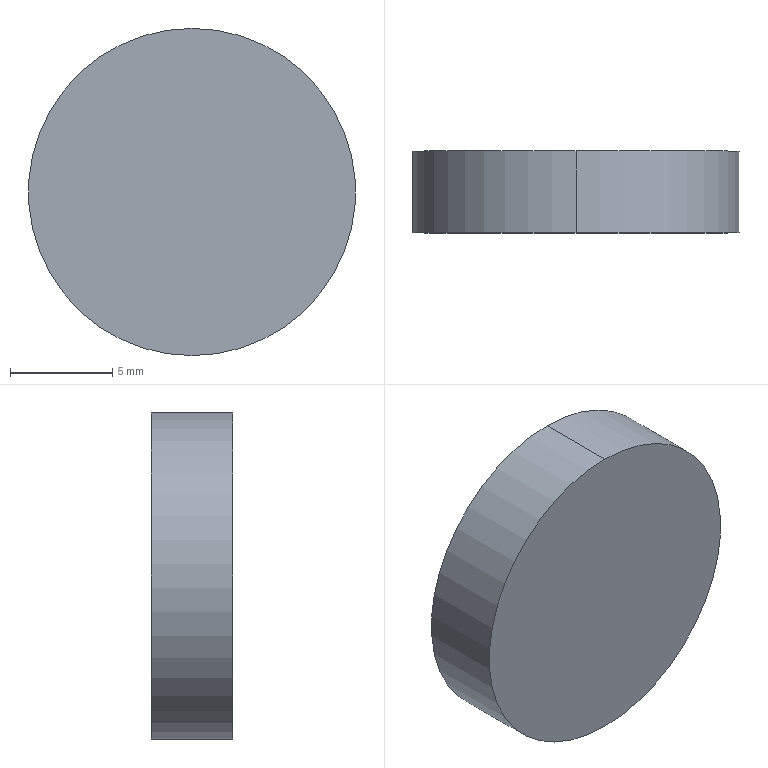Part | 1 solid | 4 faces | box 16 x 4 x 16 mm | volume 804.248 mm3 | cylinder 2 | plane 2 | commonest cylinder face diameters 16 x2
STEP:
#1=CARTESIAN_POINT('',(0.,4.,8.));
#2=VERTEX_POINT('',#1);
#3=CARTESIAN_POINT('',(0.,4.,-8.));
#4=VERTEX_POINT('',#3);
#5=CARTESIAN_POINT('',(0.,4.,0.));
#6=DIRECTION('',(0.,1.,0.));
#7=DIRECTION('',(0.,0.,1.));
#8=AXIS2_PLACEMENT_3D('',#5,#6,#7);
#9=CIRCLE('',#8,8.);
#10=EDGE_CURVE('',#2,#4,#9,.T.);
#11=ORIENTED_EDGE('',*,*,#10,.F.);
#12=CARTESIAN_POINT('',(0.,0.,8.));
#13=VERTEX_POINT('',#12);
#14=CARTESIAN_POINT('',(0.,4.,8.));
#15=DIRECTION('',(0.,-1.,0.));
#16=VECTOR('',#15,1000.);
#17=LINE('',#14,#16);
#18=EDGE_CURVE('',#2,#13,#17,.T.);
#19=ORIENTED_EDGE('',*,*,#18,.T.);
#20=CARTESIAN_POINT('',(0.,0.,-8.));
#21=VERTEX_POINT('',#20);
#22=CARTESIAN_POINT('',(0.,0.,0.));
#23=DIRECTION('',(0.,1.,0.));
#24=DIRECTION('',(0.,0.,1.));
#25=AXIS2_PLACEMENT_3D('',#22,#23,#24);
#26=CIRCLE('',#25,8.);
#27=EDGE_CURVE('',#13,#21,#26,.T.);
#28=ORIENTED_EDGE('',*,*,#27,.T.);
#29=CARTESIAN_POINT('',(0.,4.,-8.));
#30=DIRECTION('',(0.,-1.,0.));
#31=VECTOR('',#30,1000.);
#32=LINE('',#29,#31);
#33=EDGE_CURVE('',#4,#21,#32,.T.);
#34=ORIENTED_EDGE('',*,*,#33,.F.);
#35=EDGE_LOOP('',(#11,#19,#28,#34));
#36=FACE_OUTER_BOUND('',#35,.T.);
#37=CARTESIAN_POINT('',(0.,4.,0.));
#38=DIRECTION('',(0.,-1.,0.));
#39=DIRECTION('',(0.,0.,-1.));
#40=AXIS2_PLACEMENT_3D('',#37,#38,#39);
#41=CYLINDRICAL_SURFACE('',#40,8.);
#42=ADVANCED_FACE('',(#36),#41,.T.);
#43=ORIENTED_EDGE('',*,*,#18,.F.);
#44=CARTESIAN_POINT('',(0.,4.,0.));
#45=DIRECTION('',(0.,1.,0.));
#46=DIRECTION('',(0.,0.,1.));
#47=AXIS2_PLACEMENT_3D('',#44,#45,#46);
#48=CIRCLE('',#47,8.);
#49=EDGE_CURVE('',#4,#2,#48,.T.);
#50=ORIENTED_EDGE('',*,*,#49,.F.);
#51=ORIENTED_EDGE('',*,*,#33,.T.);
#52=CARTESIAN_POINT('',(0.,0.,0.));
#53=DIRECTION('',(0.,1.,0.));
#54=DIRECTION('',(0.,0.,1.));
#55=AXIS2_PLACEMENT_3D('',#52,#53,#54);
#56=CIRCLE('',#55,8.);
#57=EDGE_CURVE('',#21,#13,#56,.T.);
#58=ORIENTED_EDGE('',*,*,#57,.T.);
#59=EDGE_LOOP('',(#43,#50,#51,#58));
#60=FACE_OUTER_BOUND('',#59,.T.);
#61=CARTESIAN_POINT('',(0.,4.,0.));
#62=DIRECTION('',(0.,-1.,0.));
#63=DIRECTION('',(0.,0.,-1.));
#64=AXIS2_PLACEMENT_3D('',#61,#62,#63);
#65=CYLINDRICAL_SURFACE('',#64,8.);
#66=ADVANCED_FACE('',(#60),#65,.T.);
#67=ORIENTED_EDGE('',*,*,#49,.T.);
#68=ORIENTED_EDGE('',*,*,#10,.T.);
#69=EDGE_LOOP('',(#67,#68));
#70=FACE_OUTER_BOUND('',#69,.T.);
#71=CARTESIAN_POINT('',(0.,4.,0.));
#72=DIRECTION('',(0.,1.,0.));
#73=DIRECTION('',(1.,0.,0.));
#74=AXIS2_PLACEMENT_3D('',#71,#72,#73);
#75=PLANE('',#74);
#76=ADVANCED_FACE('',(#70),#75,.T.);
#77=ORIENTED_EDGE('',*,*,#57,.F.);
#78=ORIENTED_EDGE('',*,*,#27,.F.);
#79=EDGE_LOOP('',(#77,#78));
#80=FACE_OUTER_BOUND('',#79,.T.);
#81=CARTESIAN_POINT('',(0.,0.,0.));
#82=DIRECTION('',(0.,1.,0.));
#83=DIRECTION('',(1.,0.,0.));
#84=AXIS2_PLACEMENT_3D('',#81,#82,#83);
#85=PLANE('',#84);
#86=ADVANCED_FACE('',(#80),#85,.F.);
#87=CLOSED_SHELL('',(#42,#66,#76,#86));
#88=MANIFOLD_SOLID_BREP('',#87);
#89=CARTESIAN_POINT('',(0.,0.,0.));
#90=DIRECTION('',(0.,0.,1.));
#91=DIRECTION('',(1.,0.,0.));
#92=AXIS2_PLACEMENT_3D('',#89,#90,#91);
#93=(LENGTH_UNIT()NAMED_UNIT(*)SI_UNIT(.MILLI.,.METRE.));
#94=UNCERTAINTY_MEASURE_WITH_UNIT(LENGTH_MEASURE(0.00001),#93,'','');
#95=(NAMED_UNIT(*)PLANE_ANGLE_UNIT()SI_UNIT($,.RADIAN.));
#96=(NAMED_UNIT(*)SI_UNIT($,.STERADIAN.)SOLID_ANGLE_UNIT());
#97=(GEOMETRIC_REPRESENTATION_CONTEXT(3)GLOBAL_UNCERTAINTY_ASSIGNED_CONTEXT((#94))GLOBAL_UNIT_ASSIGNED_CONTEXT((#93,#95,#96))REPRESENTATION_CONTEXT('',''));
#98=ADVANCED_BREP_SHAPE_REPRESENTATION('',(#88,#92),#97);